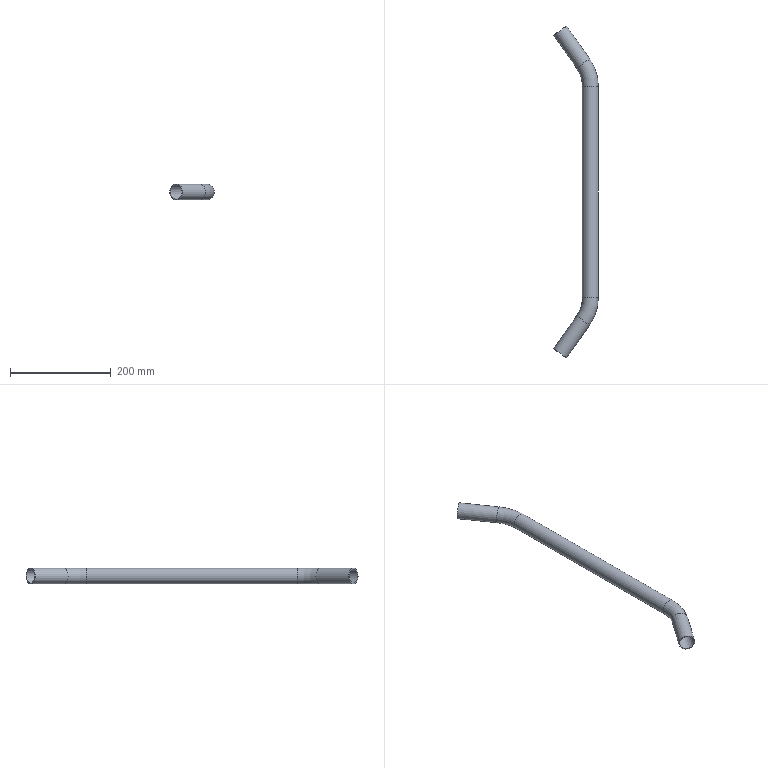Part | STEP file | 7101203 | 1 solid | 12 faces | box 89.278 x 660.628 x 31.8 mm | volume 96707 mm3 | cylinder 6 | torus 4 | plane 2 | commonest cylinder face diameters 28.8 x3 31.8 x3
STEP:
#1=CARTESIAN_POINT('',(0.,0.,0.));
#2=DIRECTION('',(0.,0.,1.));
#3=DIRECTION('',(1.,0.,0.));
#4=AXIS2_PLACEMENT_3D('',#1,#2,#3);
#5=CARTESIAN_POINT('',(-27.492,246.542,0.));
#6=VERTEX_POINT('',#5);
#7=CARTESIAN_POINT('',(-14.468,255.662,0.));
#8=DIRECTION('',(-0.5736,0.8192,0.));
#9=DIRECTION('',(-0.8192,-0.5736,0.));
#10=AXIS2_PLACEMENT_3D('',#7,#8,#9);
#11=CIRCLE('',#10,15.9);
#12=CARTESIAN_POINT('',(-14.468,255.662,0.));
#13=DIRECTION('',(-0.5736,0.8192,0.));
#14=DIRECTION('',(-0.8192,-0.5736,0.));
#15=AXIS2_PLACEMENT_3D('',#12,#13,#14);
#16=CYLINDRICAL_SURFACE('',#15,15.9);
#17=CARTESIAN_POINT('',(0.,0.));
#18=DIRECTION('',(1.,0.));
#19=VECTOR('',#18,1.);
#20=LINE('',#17,#19);
#21=(GEOMETRIC_REPRESENTATION_CONTEXT(2)PARAMETRIC_REPRESENTATION_CONTEXT()REPRESENTATION_CONTEXT('',''));
#22=DEFINITIONAL_REPRESENTATION('',(#20),#21);
#23=PCURVE('',#16,#22);
#24=CARTESIAN_POINT('',(-80.,209.776,0.));
#25=DIRECTION('',(0.,0.,1.));
#26=DIRECTION('',(1.,0.,0.));
#27=AXIS2_PLACEMENT_3D('',#24,#25,#26);
#28=TOROIDAL_SURFACE('',#27,80.,15.9);
#29=CARTESIAN_POINT('',(6.894,9.425));
#30=DIRECTION('',(0.,-1.));
#31=VECTOR('',#30,1.);
#32=LINE('',#29,#31);
#33=(GEOMETRIC_REPRESENTATION_CONTEXT(2)PARAMETRIC_REPRESENTATION_CONTEXT()REPRESENTATION_CONTEXT('',''));
#34=DEFINITIONAL_REPRESENTATION('',(#32),#33);
#35=PCURVE('',#28,#34);
#36=SURFACE_CURVE('',#11,(#23,#35),.PCURVE_S1.);
#37=EDGE_CURVE('',#6,#6,#36,.T.);
#38=ORIENTED_EDGE('',*,*,#37,.T.);
#39=CARTESIAN_POINT('',(-73.378,312.075,0.));
#40=VERTEX_POINT('',#39);
#41=CARTESIAN_POINT('',(-27.492,246.542,0.));
#42=CARTESIAN_POINT('',(-73.378,312.075,0.));
#43=B_SPLINE_CURVE_WITH_KNOTS('',1,(#41,#42),.UNSPECIFIED.,.F.,.F.,(2,2),(0.,80.),.PIECEWISE_BEZIER_KNOTS.);
#44=CARTESIAN_POINT('',(6.283,0.));
#45=DIRECTION('',(0.,1.));
#46=VECTOR('',#45,1.);
#47=LINE('',#44,#46);
#48=(GEOMETRIC_REPRESENTATION_CONTEXT(2)PARAMETRIC_REPRESENTATION_CONTEXT()REPRESENTATION_CONTEXT('',''));
#49=DEFINITIONAL_REPRESENTATION('',(#47),#48);
#50=PCURVE('',#16,#49);
#51=CARTESIAN_POINT('',(0.,0.));
#52=DIRECTION('',(0.,1.));
#53=VECTOR('',#52,1.);
#54=LINE('',#51,#53);
#55=(GEOMETRIC_REPRESENTATION_CONTEXT(2)PARAMETRIC_REPRESENTATION_CONTEXT()REPRESENTATION_CONTEXT('',''));
#56=DEFINITIONAL_REPRESENTATION('',(#54),#55);
#57=PCURVE('',#16,#56);
#58=SEAM_CURVE('',#43,(#50,#57),.PCURVE_S1.);
#59=EDGE_CURVE('',#6,#40,#58,.T.);
#60=ORIENTED_EDGE('',*,*,#59,.T.);
#61=CARTESIAN_POINT('',(-60.354,321.194,0.));
#62=DIRECTION('',(-0.5736,0.8192,0.));
#63=DIRECTION('',(-0.8192,-0.5736,0.));
#64=AXIS2_PLACEMENT_3D('',#61,#62,#63);
#65=CIRCLE('',#64,15.9);
#66=CARTESIAN_POINT('',(0.,80.));
#67=DIRECTION('',(1.,0.));
#68=VECTOR('',#67,1.);
#69=LINE('',#66,#68);
#70=(GEOMETRIC_REPRESENTATION_CONTEXT(2)PARAMETRIC_REPRESENTATION_CONTEXT()REPRESENTATION_CONTEXT('',''));
#71=DEFINITIONAL_REPRESENTATION('',(#69),#70);
#72=PCURVE('',#16,#71);
#73=CARTESIAN_POINT('',(-60.354,321.194,0.));
#74=DIRECTION('',(-0.5736,0.8192,0.));
#75=DIRECTION('',(-0.8192,-0.5736,0.));
#76=AXIS2_PLACEMENT_3D('',#73,#74,#75);
#77=PLANE('',#76);
#78=CARTESIAN_POINT('',(0.,0.));
#79=DIRECTION('',(1.,0.));
#80=AXIS2_PLACEMENT_2D('',#78,#79);
#81=CIRCLE('',#80,15.9);
#82=(GEOMETRIC_REPRESENTATION_CONTEXT(2)PARAMETRIC_REPRESENTATION_CONTEXT()REPRESENTATION_CONTEXT('',''));
#83=DEFINITIONAL_REPRESENTATION('',(#81),#82);
#84=PCURVE('',#77,#83);
#85=SURFACE_CURVE('',#65,(#72,#84),.PCURVE_S1.);
#86=EDGE_CURVE('',#40,#40,#85,.T.);
#87=ORIENTED_EDGE('',*,*,#86,.F.);
#88=ORIENTED_EDGE('',*,*,#59,.F.);
#89=EDGE_LOOP('',(#38,#60,#87,#88));
#90=FACE_BOUND('',#89,.T.);
#91=ADVANCED_FACE('',(#90),#16,.T.);
#92=CARTESIAN_POINT('',(-26.264,247.403,0.));
#93=VERTEX_POINT('',#92);
#94=CARTESIAN_POINT('',(-14.468,255.662,0.));
#95=DIRECTION('',(-0.5736,0.8192,0.));
#96=DIRECTION('',(-0.8192,-0.5736,0.));
#97=AXIS2_PLACEMENT_3D('',#94,#95,#96);
#98=CIRCLE('',#97,14.4);
#99=CARTESIAN_POINT('',(-14.468,255.662,0.));
#100=DIRECTION('',(-0.5736,0.8192,0.));
#101=DIRECTION('',(-0.8192,-0.5736,0.));
#102=AXIS2_PLACEMENT_3D('',#99,#100,#101);
#103=CYLINDRICAL_SURFACE('',#102,14.4);
#104=CARTESIAN_POINT('',(0.,0.));
#105=DIRECTION('',(1.,0.));
#106=VECTOR('',#105,1.);
#107=LINE('',#104,#106);
#108=(GEOMETRIC_REPRESENTATION_CONTEXT(2)PARAMETRIC_REPRESENTATION_CONTEXT()REPRESENTATION_CONTEXT('',''));
#109=DEFINITIONAL_REPRESENTATION('',(#107),#108);
#110=PCURVE('',#103,#109);
#111=CARTESIAN_POINT('',(-80.,209.776,0.));
#112=DIRECTION('',(0.,0.,1.));
#113=DIRECTION('',(1.,0.,0.));
#114=AXIS2_PLACEMENT_3D('',#111,#112,#113);
#115=TOROIDAL_SURFACE('',#114,80.,14.4);
#116=CARTESIAN_POINT('',(6.894,9.425));
#117=DIRECTION('',(0.,-1.));
#118=VECTOR('',#117,1.);
#119=LINE('',#116,#118);
#120=(GEOMETRIC_REPRESENTATION_CONTEXT(2)PARAMETRIC_REPRESENTATION_CONTEXT()REPRESENTATION_CONTEXT('',''));
#121=DEFINITIONAL_REPRESENTATION('',(#119),#120);
#122=PCURVE('',#115,#121);
#123=SURFACE_CURVE('',#98,(#110,#122),.PCURVE_S1.);
#124=EDGE_CURVE('',#93,#93,#123,.T.);
#125=ORIENTED_EDGE('',*,*,#124,.T.);
#126=CARTESIAN_POINT('',(-72.15,312.935,0.));
#127=VERTEX_POINT('',#126);
#128=CARTESIAN_POINT('',(-26.264,247.403,0.));
#129=CARTESIAN_POINT('',(-72.15,312.935,0.));
#130=B_SPLINE_CURVE_WITH_KNOTS('',1,(#128,#129),.UNSPECIFIED.,.F.,.F.,(2,2),(0.,80.),.PIECEWISE_BEZIER_KNOTS.);
#131=CARTESIAN_POINT('',(6.283,0.));
#132=DIRECTION('',(0.,1.));
#133=VECTOR('',#132,1.);
#134=LINE('',#131,#133);
#135=(GEOMETRIC_REPRESENTATION_CONTEXT(2)PARAMETRIC_REPRESENTATION_CONTEXT()REPRESENTATION_CONTEXT('',''));
#136=DEFINITIONAL_REPRESENTATION('',(#134),#135);
#137=PCURVE('',#103,#136);
#138=CARTESIAN_POINT('',(0.,0.));
#139=DIRECTION('',(0.,1.));
#140=VECTOR('',#139,1.);
#141=LINE('',#138,#140);
#142=(GEOMETRIC_REPRESENTATION_CONTEXT(2)PARAMETRIC_REPRESENTATION_CONTEXT()REPRESENTATION_CONTEXT('',''));
#143=DEFINITIONAL_REPRESENTATION('',(#141),#142);
#144=PCURVE('',#103,#143);
#145=SEAM_CURVE('',#130,(#137,#144),.PCURVE_S1.);
#146=EDGE_CURVE('',#93,#127,#145,.T.);
#147=ORIENTED_EDGE('',*,*,#146,.T.);
#148=CARTESIAN_POINT('',(-60.354,321.194,0.));
#149=DIRECTION('',(-0.5736,0.8192,0.));
#150=DIRECTION('',(-0.8192,-0.5736,0.));
#151=AXIS2_PLACEMENT_3D('',#148,#149,#150);
#152=CIRCLE('',#151,14.4);
#153=CARTESIAN_POINT('',(0.,80.));
#154=DIRECTION('',(1.,0.));
#155=VECTOR('',#154,1.);
#156=LINE('',#153,#155);
#157=(GEOMETRIC_REPRESENTATION_CONTEXT(2)PARAMETRIC_REPRESENTATION_CONTEXT()REPRESENTATION_CONTEXT('',''));
#158=DEFINITIONAL_REPRESENTATION('',(#156),#157);
#159=PCURVE('',#103,#158);
#160=CARTESIAN_POINT('',(0.,0.));
#161=DIRECTION('',(1.,0.));
#162=AXIS2_PLACEMENT_2D('',#160,#161);
#163=CIRCLE('',#162,14.4);
#164=(GEOMETRIC_REPRESENTATION_CONTEXT(2)PARAMETRIC_REPRESENTATION_CONTEXT()REPRESENTATION_CONTEXT('',''));
#165=DEFINITIONAL_REPRESENTATION('',(#163),#164);
#166=PCURVE('',#77,#165);
#167=SURFACE_CURVE('',#152,(#159,#166),.PCURVE_S1.);
#168=EDGE_CURVE('',#127,#127,#167,.T.);
#169=ORIENTED_EDGE('',*,*,#168,.F.);
#170=ORIENTED_EDGE('',*,*,#146,.F.);
#171=EDGE_LOOP('',(#125,#147,#169,#170));
#172=FACE_BOUND('',#171,.F.);
#173=ADVANCED_FACE('',(#172),#103,.F.);
#174=CARTESIAN_POINT('',(-15.9,209.776,0.));
#175=VERTEX_POINT('',#174);
#176=CARTESIAN_POINT('',(0.,209.776,0.));
#177=DIRECTION('',(0.,1.,0.));
#178=DIRECTION('',(-1.,0.,0.));
#179=AXIS2_PLACEMENT_3D('',#176,#177,#178);
#180=CIRCLE('',#179,15.9);
#181=CARTESIAN_POINT('',(6.283,9.425));
#182=DIRECTION('',(0.,-1.));
#183=VECTOR('',#182,1.);
#184=LINE('',#181,#183);
#185=(GEOMETRIC_REPRESENTATION_CONTEXT(2)PARAMETRIC_REPRESENTATION_CONTEXT()REPRESENTATION_CONTEXT('',''));
#186=DEFINITIONAL_REPRESENTATION('',(#184),#185);
#187=PCURVE('',#28,#186);
#188=CARTESIAN_POINT('',(0.,-209.776,0.));
#189=DIRECTION('',(0.,1.,0.));
#190=DIRECTION('',(-1.,0.,0.));
#191=AXIS2_PLACEMENT_3D('',#188,#189,#190);
#192=CYLINDRICAL_SURFACE('',#191,15.9);
#193=CARTESIAN_POINT('',(0.,419.552));
#194=DIRECTION('',(1.,0.));
#195=VECTOR('',#194,1.);
#196=LINE('',#193,#195);
#197=(GEOMETRIC_REPRESENTATION_CONTEXT(2)PARAMETRIC_REPRESENTATION_CONTEXT()REPRESENTATION_CONTEXT('',''));
#198=DEFINITIONAL_REPRESENTATION('',(#196),#197);
#199=PCURVE('',#192,#198);
#200=SURFACE_CURVE('',#180,(#187,#199),.PCURVE_S1.);
#201=EDGE_CURVE('',#175,#175,#200,.T.);
#202=ORIENTED_EDGE('',*,*,#201,.T.);
#203=CARTESIAN_POINT('',(-15.9,209.776,0.));
#204=CARTESIAN_POINT('',(-15.9,216.323,0.));
#205=CARTESIAN_POINT('',(-16.701,222.844,0.));
#206=CARTESIAN_POINT('',(-18.294,229.232,0.));
#207=CARTESIAN_POINT('',(-20.653,235.378,0.));
#208=CARTESIAN_POINT('',(-23.737,241.18,0.));
#209=CARTESIAN_POINT('',(-27.492,246.542,0.));
#210=(BOUNDED_CURVE()B_SPLINE_CURVE(6,(#203,#204,#205,#206,#207,#208,#209),.UNSPECIFIED.,.F.,.F.)B_SPLINE_CURVE_WITH_KNOTS((7,7),(6.283,6.894),.PIECEWISE_BEZIER_KNOTS.)CURVE()GEOMETRIC_REPRESENTATION_ITEM()RATIONAL_B_SPLINE_CURVE((1.005,1.002,0.9997,0.9991,0.9997,1.002,1.005))REPRESENTATION_ITEM(''));
#211=CARTESIAN_POINT('',(0.,3.142));
#212=DIRECTION('',(1.,0.));
#213=VECTOR('',#212,1.);
#214=LINE('',#211,#213);
#215=(GEOMETRIC_REPRESENTATION_CONTEXT(2)PARAMETRIC_REPRESENTATION_CONTEXT()REPRESENTATION_CONTEXT('',''));
#216=DEFINITIONAL_REPRESENTATION('',(#214),#215);
#217=PCURVE('',#28,#216);
#218=CARTESIAN_POINT('',(0.,9.425));
#219=DIRECTION('',(1.,0.));
#220=VECTOR('',#219,1.);
#221=LINE('',#218,#220);
#222=(GEOMETRIC_REPRESENTATION_CONTEXT(2)PARAMETRIC_REPRESENTATION_CONTEXT()REPRESENTATION_CONTEXT('',''));
#223=DEFINITIONAL_REPRESENTATION('',(#221),#222);
#224=PCURVE('',#28,#223);
#225=SEAM_CURVE('',#210,(#217,#224),.PCURVE_S1.);
#226=EDGE_CURVE('',#175,#6,#225,.T.);
#227=ORIENTED_EDGE('',*,*,#226,.T.);
#228=ORIENTED_EDGE('',*,*,#37,.F.);
#229=ORIENTED_EDGE('',*,*,#226,.F.);
#230=EDGE_LOOP('',(#202,#227,#228,#229));
#231=FACE_BOUND('',#230,.T.);
#232=ADVANCED_FACE('',(#231),#28,.T.);
#233=CARTESIAN_POINT('',(-14.4,209.776,0.));
#234=VERTEX_POINT('',#233);
#235=CARTESIAN_POINT('',(0.,209.776,0.));
#236=DIRECTION('',(0.,1.,0.));
#237=DIRECTION('',(-1.,0.,0.));
#238=AXIS2_PLACEMENT_3D('',#235,#236,#237);
#239=CIRCLE('',#238,14.4);
#240=CARTESIAN_POINT('',(6.283,9.425));
#241=DIRECTION('',(0.,-1.));
#242=VECTOR('',#241,1.);
#243=LINE('',#240,#242);
#244=(GEOMETRIC_REPRESENTATION_CONTEXT(2)PARAMETRIC_REPRESENTATION_CONTEXT()REPRESENTATION_CONTEXT('',''));
#245=DEFINITIONAL_REPRESENTATION('',(#243),#244);
#246=PCURVE('',#115,#245);
#247=CARTESIAN_POINT('',(0.,-209.776,0.));
#248=DIRECTION('',(0.,1.,0.));
#249=DIRECTION('',(-1.,0.,0.));
#250=AXIS2_PLACEMENT_3D('',#247,#248,#249);
#251=CYLINDRICAL_SURFACE('',#250,14.4);
#252=CARTESIAN_POINT('',(0.,419.552));
#253=DIRECTION('',(1.,0.));
#254=VECTOR('',#253,1.);
#255=LINE('',#252,#254);
#256=(GEOMETRIC_REPRESENTATION_CONTEXT(2)PARAMETRIC_REPRESENTATION_CONTEXT()REPRESENTATION_CONTEXT('',''));
#257=DEFINITIONAL_REPRESENTATION('',(#255),#256);
#258=PCURVE('',#251,#257);
#259=SURFACE_CURVE('',#239,(#246,#258),.PCURVE_S1.);
#260=EDGE_CURVE('',#234,#234,#259,.T.);
#261=ORIENTED_EDGE('',*,*,#260,.T.);
#262=CARTESIAN_POINT('',(-14.4,209.776,0.));
#263=CARTESIAN_POINT('',(-14.4,216.476,0.));
#264=CARTESIAN_POINT('',(-15.22,223.15,0.));
#265=CARTESIAN_POINT('',(-16.85,229.687,0.));
#266=CARTESIAN_POINT('',(-19.264,235.977,0.));
#267=CARTESIAN_POINT('',(-22.421,241.915,0.));
#268=CARTESIAN_POINT('',(-26.264,247.403,0.));
#269=(BOUNDED_CURVE()B_SPLINE_CURVE(6,(#262,#263,#264,#265,#266,#267,#268),.UNSPECIFIED.,.F.,.F.)B_SPLINE_CURVE_WITH_KNOTS((7,7),(6.283,6.894),.PIECEWISE_BEZIER_KNOTS.)CURVE()GEOMETRIC_REPRESENTATION_ITEM()RATIONAL_B_SPLINE_CURVE((1.005,1.002,0.9997,0.9991,0.9997,1.002,1.005))REPRESENTATION_ITEM(''));
#270=CARTESIAN_POINT('',(0.,3.142));
#271=DIRECTION('',(1.,0.));
#272=VECTOR('',#271,1.);
#273=LINE('',#270,#272);
#274=(GEOMETRIC_REPRESENTATION_CONTEXT(2)PARAMETRIC_REPRESENTATION_CONTEXT()REPRESENTATION_CONTEXT('',''));
#275=DEFINITIONAL_REPRESENTATION('',(#273),#274);
#276=PCURVE('',#115,#275);
#277=CARTESIAN_POINT('',(0.,9.425));
#278=DIRECTION('',(1.,0.));
#279=VECTOR('',#278,1.);
#280=LINE('',#277,#279);
#281=(GEOMETRIC_REPRESENTATION_CONTEXT(2)PARAMETRIC_REPRESENTATION_CONTEXT()REPRESENTATION_CONTEXT('',''));
#282=DEFINITIONAL_REPRESENTATION('',(#280),#281);
#283=PCURVE('',#115,#282);
#284=SEAM_CURVE('',#269,(#276,#283),.PCURVE_S1.);
#285=EDGE_CURVE('',#234,#93,#284,.T.);
#286=ORIENTED_EDGE('',*,*,#285,.T.);
#287=ORIENTED_EDGE('',*,*,#124,.F.);
#288=ORIENTED_EDGE('',*,*,#285,.F.);
#289=EDGE_LOOP('',(#261,#286,#287,#288));
#290=FACE_BOUND('',#289,.F.);
#291=ADVANCED_FACE('',(#290),#115,.F.);
#292=CARTESIAN_POINT('',(-15.9,-209.776,0.));
#293=VERTEX_POINT('',#292);
#294=CARTESIAN_POINT('',(0.,-209.776,0.));
#295=DIRECTION('',(0.,1.,0.));
#296=DIRECTION('',(-1.,0.,0.));
#297=AXIS2_PLACEMENT_3D('',#294,#295,#296);
#298=CIRCLE('',#297,15.9);
#299=CARTESIAN_POINT('',(0.,0.));
#300=DIRECTION('',(1.,0.));
#301=VECTOR('',#300,1.);
#302=LINE('',#299,#301);
#303=(GEOMETRIC_REPRESENTATION_CONTEXT(2)PARAMETRIC_REPRESENTATION_CONTEXT()REPRESENTATION_CONTEXT('',''));
#304=DEFINITIONAL_REPRESENTATION('',(#302),#303);
#305=PCURVE('',#192,#304);
#306=CARTESIAN_POINT('',(-80.,-209.776,0.));
#307=DIRECTION('',(0.,0.,1.));
#308=DIRECTION('',(1.,0.,0.));
#309=AXIS2_PLACEMENT_3D('',#306,#307,#308);
#310=TOROIDAL_SURFACE('',#309,80.,15.9);
#311=CARTESIAN_POINT('',(6.283,9.425));
#312=DIRECTION('',(0.,-1.));
#313=VECTOR('',#312,1.);
#314=LINE('',#311,#313);
#315=(GEOMETRIC_REPRESENTATION_CONTEXT(2)PARAMETRIC_REPRESENTATION_CONTEXT()REPRESENTATION_CONTEXT('',''));
#316=DEFINITIONAL_REPRESENTATION('',(#314),#315);
#317=PCURVE('',#310,#316);
#318=SURFACE_CURVE('',#298,(#305,#317),.PCURVE_S1.);
#319=EDGE_CURVE('',#293,#293,#318,.T.);
#320=ORIENTED_EDGE('',*,*,#319,.T.);
#321=CARTESIAN_POINT('',(-15.9,-209.776,0.));
#322=CARTESIAN_POINT('',(-15.9,209.776,0.));
#323=B_SPLINE_CURVE_WITH_KNOTS('',1,(#321,#322),.UNSPECIFIED.,.F.,.F.,(2,2),(0.,419.552),.PIECEWISE_BEZIER_KNOTS.);
#324=CARTESIAN_POINT('',(6.283,0.));
#325=DIRECTION('',(0.,1.));
#326=VECTOR('',#325,1.);
#327=LINE('',#324,#326);
#328=(GEOMETRIC_REPRESENTATION_CONTEXT(2)PARAMETRIC_REPRESENTATION_CONTEXT()REPRESENTATION_CONTEXT('',''));
#329=DEFINITIONAL_REPRESENTATION('',(#327),#328);
#330=PCURVE('',#192,#329);
#331=CARTESIAN_POINT('',(0.,0.));
#332=DIRECTION('',(0.,1.));
#333=VECTOR('',#332,1.);
#334=LINE('',#331,#333);
#335=(GEOMETRIC_REPRESENTATION_CONTEXT(2)PARAMETRIC_REPRESENTATION_CONTEXT()REPRESENTATION_CONTEXT('',''));
#336=DEFINITIONAL_REPRESENTATION('',(#334),#335);
#337=PCURVE('',#192,#336);
#338=SEAM_CURVE('',#323,(#330,#337),.PCURVE_S1.);
#339=EDGE_CURVE('',#293,#175,#338,.T.);
#340=ORIENTED_EDGE('',*,*,#339,.T.);
#341=ORIENTED_EDGE('',*,*,#201,.F.);
#342=ORIENTED_EDGE('',*,*,#339,.F.);
#343=EDGE_LOOP('',(#320,#340,#341,#342));
#344=FACE_BOUND('',#343,.T.);
#345=ADVANCED_FACE('',(#344),#192,.T.);
#346=CARTESIAN_POINT('',(-14.4,-209.776,0.));
#347=VERTEX_POINT('',#346);
#348=CARTESIAN_POINT('',(0.,-209.776,0.));
#349=DIRECTION('',(0.,1.,0.));
#350=DIRECTION('',(-1.,0.,0.));
#351=AXIS2_PLACEMENT_3D('',#348,#349,#350);
#352=CIRCLE('',#351,14.4);
#353=CARTESIAN_POINT('',(0.,0.));
#354=DIRECTION('',(1.,0.));
#355=VECTOR('',#354,1.);
#356=LINE('',#353,#355);
#357=(GEOMETRIC_REPRESENTATION_CONTEXT(2)PARAMETRIC_REPRESENTATION_CONTEXT()REPRESENTATION_CONTEXT('',''));
#358=DEFINITIONAL_REPRESENTATION('',(#356),#357);
#359=PCURVE('',#251,#358);
#360=CARTESIAN_POINT('',(-80.,-209.776,0.));
#361=DIRECTION('',(0.,0.,1.));
#362=DIRECTION('',(1.,0.,0.));
#363=AXIS2_PLACEMENT_3D('',#360,#361,#362);
#364=TOROIDAL_SURFACE('',#363,80.,14.4);
#365=CARTESIAN_POINT('',(6.283,9.425));
#366=DIRECTION('',(0.,-1.));
#367=VECTOR('',#366,1.);
#368=LINE('',#365,#367);
#369=(GEOMETRIC_REPRESENTATION_CONTEXT(2)PARAMETRIC_REPRESENTATION_CONTEXT()REPRESENTATION_CONTEXT('',''));
#370=DEFINITIONAL_REPRESENTATION('',(#368),#369);
#371=PCURVE('',#364,#370);
#372=SURFACE_CURVE('',#352,(#359,#371),.PCURVE_S1.);
#373=EDGE_CURVE('',#347,#347,#372,.T.);
#374=ORIENTED_EDGE('',*,*,#373,.T.);
#375=CARTESIAN_POINT('',(-14.4,-209.776,0.));
#376=CARTESIAN_POINT('',(-14.4,209.776,0.));
#377=B_SPLINE_CURVE_WITH_KNOTS('',1,(#375,#376),.UNSPECIFIED.,.F.,.F.,(2,2),(0.,419.552),.PIECEWISE_BEZIER_KNOTS.);
#378=CARTESIAN_POINT('',(6.283,0.));
#379=DIRECTION('',(0.,1.));
#380=VECTOR('',#379,1.);
#381=LINE('',#378,#380);
#382=(GEOMETRIC_REPRESENTATION_CONTEXT(2)PARAMETRIC_REPRESENTATION_CONTEXT()REPRESENTATION_CONTEXT('',''));
#383=DEFINITIONAL_REPRESENTATION('',(#381),#382);
#384=PCURVE('',#251,#383);
#385=CARTESIAN_POINT('',(0.,0.));
#386=DIRECTION('',(0.,1.));
#387=VECTOR('',#386,1.);
#388=LINE('',#385,#387);
#389=(GEOMETRIC_REPRESENTATION_CONTEXT(2)PARAMETRIC_REPRESENTATION_CONTEXT()REPRESENTATION_CONTEXT('',''));
#390=DEFINITIONAL_REPRESENTATION('',(#388),#389);
#391=PCURVE('',#251,#390);
#392=SEAM_CURVE('',#377,(#384,#391),.PCURVE_S1.);
#393=EDGE_CURVE('',#347,#234,#392,.T.);
#394=ORIENTED_EDGE('',*,*,#393,.T.);
#395=ORIENTED_EDGE('',*,*,#260,.F.);
#396=ORIENTED_EDGE('',*,*,#393,.F.);
#397=EDGE_LOOP('',(#374,#394,#395,#396));
#398=FACE_BOUND('',#397,.F.);
#399=ADVANCED_FACE('',(#398),#251,.F.);
#400=CARTESIAN_POINT('',(-27.492,-246.542,0.));
#401=VERTEX_POINT('',#400);
#402=CARTESIAN_POINT('',(-14.468,-255.662,0.));
#403=DIRECTION('',(0.5736,0.8192,0.));
#404=DIRECTION('',(-0.8192,0.5736,0.));
#405=AXIS2_PLACEMENT_3D('',#402,#403,#404);
#406=CIRCLE('',#405,15.9);
#407=CARTESIAN_POINT('',(5.672,9.425));
#408=DIRECTION('',(0.,-1.));
#409=VECTOR('',#408,1.);
#410=LINE('',#407,#409);
#411=(GEOMETRIC_REPRESENTATION_CONTEXT(2)PARAMETRIC_REPRESENTATION_CONTEXT()REPRESENTATION_CONTEXT('',''));
#412=DEFINITIONAL_REPRESENTATION('',(#410),#411);
#413=PCURVE('',#310,#412);
#414=CARTESIAN_POINT('',(-14.468,-255.662,0.));
#415=DIRECTION('',(-0.5736,-0.8192,0.));
#416=DIRECTION('',(0.8192,-0.5736,0.));
#417=AXIS2_PLACEMENT_3D('',#414,#415,#416);
#418=CYLINDRICAL_SURFACE('',#417,15.9);
#419=CARTESIAN_POINT('',(9.425,0.));
#420=DIRECTION('',(-1.,0.));
#421=VECTOR('',#420,1.);
#422=LINE('',#419,#421);
#423=(GEOMETRIC_REPRESENTATION_CONTEXT(2)PARAMETRIC_REPRESENTATION_CONTEXT()REPRESENTATION_CONTEXT('',''));
#424=DEFINITIONAL_REPRESENTATION('',(#422),#423);
#425=PCURVE('',#418,#424);
#426=SURFACE_CURVE('',#406,(#413,#425),.PCURVE_S1.);
#427=EDGE_CURVE('',#401,#401,#426,.T.);
#428=ORIENTED_EDGE('',*,*,#427,.T.);
#429=CARTESIAN_POINT('',(-27.492,-246.542,0.));
#430=CARTESIAN_POINT('',(-23.737,-241.18,0.));
#431=CARTESIAN_POINT('',(-20.653,-235.378,0.));
#432=CARTESIAN_POINT('',(-18.294,-229.232,0.));
#433=CARTESIAN_POINT('',(-16.701,-222.844,0.));
#434=CARTESIAN_POINT('',(-15.9,-216.323,0.));
#435=CARTESIAN_POINT('',(-15.9,-209.776,0.));
#436=(BOUNDED_CURVE()B_SPLINE_CURVE(6,(#429,#430,#431,#432,#433,#434,#435),.UNSPECIFIED.,.F.,.F.)B_SPLINE_CURVE_WITH_KNOTS((7,7),(5.672,6.283),.PIECEWISE_BEZIER_KNOTS.)CURVE()GEOMETRIC_REPRESENTATION_ITEM()RATIONAL_B_SPLINE_CURVE((1.005,1.002,0.9997,0.9991,0.9997,1.002,1.005))REPRESENTATION_ITEM(''));
#437=CARTESIAN_POINT('',(0.,3.142));
#438=DIRECTION('',(1.,0.));
#439=VECTOR('',#438,1.);
#440=LINE('',#437,#439);
#441=(GEOMETRIC_REPRESENTATION_CONTEXT(2)PARAMETRIC_REPRESENTATION_CONTEXT()REPRESENTATION_CONTEXT('',''));
#442=DEFINITIONAL_REPRESENTATION('',(#440),#441);
#443=PCURVE('',#310,#442);
#444=CARTESIAN_POINT('',(0.,9.425));
#445=DIRECTION('',(1.,0.));
#446=VECTOR('',#445,1.);
#447=LINE('',#444,#446);
#448=(GEOMETRIC_REPRESENTATION_CONTEXT(2)PARAMETRIC_REPRESENTATION_CONTEXT()REPRESENTATION_CONTEXT('',''));
#449=DEFINITIONAL_REPRESENTATION('',(#447),#448);
#450=PCURVE('',#310,#449);
#451=SEAM_CURVE('',#436,(#443,#450),.PCURVE_S1.);
#452=EDGE_CURVE('',#401,#293,#451,.T.);
#453=ORIENTED_EDGE('',*,*,#452,.T.);
#454=ORIENTED_EDGE('',*,*,#319,.F.);
#455=ORIENTED_EDGE('',*,*,#452,.F.);
#456=EDGE_LOOP('',(#428,#453,#454,#455));
#457=FACE_BOUND('',#456,.T.);
#458=ADVANCED_FACE('',(#457),#310,.T.);
#459=CARTESIAN_POINT('',(-26.264,-247.403,0.));
#460=VERTEX_POINT('',#459);
#461=CARTESIAN_POINT('',(-14.468,-255.662,0.));
#462=DIRECTION('',(0.5736,0.8192,0.));
#463=DIRECTION('',(-0.8192,0.5736,0.));
#464=AXIS2_PLACEMENT_3D('',#461,#462,#463);
#465=CIRCLE('',#464,14.4);
#466=CARTESIAN_POINT('',(5.672,9.425));
#467=DIRECTION('',(0.,-1.));
#468=VECTOR('',#467,1.);
#469=LINE('',#466,#468);
#470=(GEOMETRIC_REPRESENTATION_CONTEXT(2)PARAMETRIC_REPRESENTATION_CONTEXT()REPRESENTATION_CONTEXT('',''));
#471=DEFINITIONAL_REPRESENTATION('',(#469),#470);
#472=PCURVE('',#364,#471);
#473=CARTESIAN_POINT('',(-14.468,-255.662,0.));
#474=DIRECTION('',(-0.5736,-0.8192,0.));
#475=DIRECTION('',(0.8192,-0.5736,0.));
#476=AXIS2_PLACEMENT_3D('',#473,#474,#475);
#477=CYLINDRICAL_SURFACE('',#476,14.4);
#478=CARTESIAN_POINT('',(9.425,0.));
#479=DIRECTION('',(-1.,0.));
#480=VECTOR('',#479,1.);
#481=LINE('',#478,#480);
#482=(GEOMETRIC_REPRESENTATION_CONTEXT(2)PARAMETRIC_REPRESENTATION_CONTEXT()REPRESENTATION_CONTEXT('',''));
#483=DEFINITIONAL_REPRESENTATION('',(#481),#482);
#484=PCURVE('',#477,#483);
#485=SURFACE_CURVE('',#465,(#472,#484),.PCURVE_S1.);
#486=EDGE_CURVE('',#460,#460,#485,.T.);
#487=ORIENTED_EDGE('',*,*,#486,.T.);
#488=CARTESIAN_POINT('',(-26.264,-247.403,0.));
#489=CARTESIAN_POINT('',(-22.421,-241.915,0.));
#490=CARTESIAN_POINT('',(-19.264,-235.977,0.));
#491=CARTESIAN_POINT('',(-16.85,-229.687,0.));
#492=CARTESIAN_POINT('',(-15.22,-223.15,0.));
#493=CARTESIAN_POINT('',(-14.4,-216.476,0.));
#494=CARTESIAN_POINT('',(-14.4,-209.776,0.));
#495=(BOUNDED_CURVE()B_SPLINE_CURVE(6,(#488,#489,#490,#491,#492,#493,#494),.UNSPECIFIED.,.F.,.F.)B_SPLINE_CURVE_WITH_KNOTS((7,7),(5.672,6.283),.PIECEWISE_BEZIER_KNOTS.)CURVE()GEOMETRIC_REPRESENTATION_ITEM()RATIONAL_B_SPLINE_CURVE((1.005,1.002,0.9997,0.9991,0.9997,1.002,1.005))REPRESENTATION_ITEM(''));
#496=CARTESIAN_POINT('',(0.,3.142));
#497=DIRECTION('',(1.,0.));
#498=VECTOR('',#497,1.);
#499=LINE('',#496,#498);
#500=(GEOMETRIC_REPRESENTATION_CONTEXT(2)PARAMETRIC_REPRESENTATION_CONTEXT()REPRESENTATION_CONTEXT('',''));
#501=DEFINITIONAL_REPRESENTATION('',(#499),#500);
#502=PCURVE('',#364,#501);
#503=CARTESIAN_POINT('',(0.,9.425));
#504=DIRECTION('',(1.,0.));
#505=VECTOR('',#504,1.);
#506=LINE('',#503,#505);
#507=(GEOMETRIC_REPRESENTATION_CONTEXT(2)PARAMETRIC_REPRESENTATION_CONTEXT()REPRESENTATION_CONTEXT('',''));
#508=DEFINITIONAL_REPRESENTATION('',(#506),#507);
#509=PCURVE('',#364,#508);
#510=SEAM_CURVE('',#495,(#502,#509),.PCURVE_S1.);
#511=EDGE_CURVE('',#460,#347,#510,.T.);
#512=ORIENTED_EDGE('',*,*,#511,.T.);
#513=ORIENTED_EDGE('',*,*,#373,.F.);
#514=ORIENTED_EDGE('',*,*,#511,.F.);
#515=EDGE_LOOP('',(#487,#512,#513,#514));
#516=FACE_BOUND('',#515,.F.);
#517=ADVANCED_FACE('',(#516),#364,.F.);
#518=ORIENTED_EDGE('',*,*,#486,.F.);
#519=CARTESIAN_POINT('',(-72.15,-312.935,0.));
#520=VERTEX_POINT('',#519);
#521=CARTESIAN_POINT('',(-26.264,-247.403,0.));
#522=CARTESIAN_POINT('',(-72.15,-312.935,0.));
#523=B_SPLINE_CURVE_WITH_KNOTS('',1,(#521,#522),.UNSPECIFIED.,.F.,.F.,(2,2),(0.,80.),.PIECEWISE_BEZIER_KNOTS.);
#524=CARTESIAN_POINT('',(9.425,0.));
#525=DIRECTION('',(0.,1.));
#526=VECTOR('',#525,1.);
#527=LINE('',#524,#526);
#528=(GEOMETRIC_REPRESENTATION_CONTEXT(2)PARAMETRIC_REPRESENTATION_CONTEXT()REPRESENTATION_CONTEXT('',''));
#529=DEFINITIONAL_REPRESENTATION('',(#527),#528);
#530=PCURVE('',#477,#529);
#531=CARTESIAN_POINT('',(3.142,0.));
#532=DIRECTION('',(0.,1.));
#533=VECTOR('',#532,1.);
#534=LINE('',#531,#533);
#535=(GEOMETRIC_REPRESENTATION_CONTEXT(2)PARAMETRIC_REPRESENTATION_CONTEXT()REPRESENTATION_CONTEXT('',''));
#536=DEFINITIONAL_REPRESENTATION('',(#534),#535);
#537=PCURVE('',#477,#536);
#538=SEAM_CURVE('',#523,(#530,#537),.PCURVE_S1.);
#539=EDGE_CURVE('',#460,#520,#538,.T.);
#540=ORIENTED_EDGE('',*,*,#539,.T.);
#541=CARTESIAN_POINT('',(-60.354,-321.194,0.));
#542=DIRECTION('',(0.5736,0.8192,0.));
#543=DIRECTION('',(-0.8192,0.5736,0.));
#544=AXIS2_PLACEMENT_3D('',#541,#542,#543);
#545=CIRCLE('',#544,14.4);
#546=CARTESIAN_POINT('',(9.425,80.));
#547=DIRECTION('',(-1.,0.));
#548=VECTOR('',#547,1.);
#549=LINE('',#546,#548);
#550=(GEOMETRIC_REPRESENTATION_CONTEXT(2)PARAMETRIC_REPRESENTATION_CONTEXT()REPRESENTATION_CONTEXT('',''));
#551=DEFINITIONAL_REPRESENTATION('',(#549),#550);
#552=PCURVE('',#477,#551);
#553=CARTESIAN_POINT('',(-60.354,-321.194,0.));
#554=DIRECTION('',(0.5736,0.8192,0.));
#555=DIRECTION('',(-0.8192,0.5736,0.));
#556=AXIS2_PLACEMENT_3D('',#553,#554,#555);
#557=PLANE('',#556);
#558=CARTESIAN_POINT('',(0.,0.));
#559=DIRECTION('',(1.,0.));
#560=AXIS2_PLACEMENT_2D('',#558,#559);
#561=CIRCLE('',#560,14.4);
#562=(GEOMETRIC_REPRESENTATION_CONTEXT(2)PARAMETRIC_REPRESENTATION_CONTEXT()REPRESENTATION_CONTEXT('',''));
#563=DEFINITIONAL_REPRESENTATION('',(#561),#562);
#564=PCURVE('',#557,#563);
#565=SURFACE_CURVE('',#545,(#552,#564),.PCURVE_S1.);
#566=EDGE_CURVE('',#520,#520,#565,.T.);
#567=ORIENTED_EDGE('',*,*,#566,.T.);
#568=ORIENTED_EDGE('',*,*,#539,.F.);
#569=EDGE_LOOP('',(#518,#540,#567,#568));
#570=FACE_BOUND('',#569,.F.);
#571=ADVANCED_FACE('',(#570),#477,.F.);
#572=ORIENTED_EDGE('',*,*,#427,.F.);
#573=CARTESIAN_POINT('',(-73.378,-312.075,0.));
#574=VERTEX_POINT('',#573);
#575=CARTESIAN_POINT('',(-27.492,-246.542,0.));
#576=CARTESIAN_POINT('',(-73.378,-312.075,0.));
#577=B_SPLINE_CURVE_WITH_KNOTS('',1,(#575,#576),.UNSPECIFIED.,.F.,.F.,(2,2),(0.,80.),.PIECEWISE_BEZIER_KNOTS.);
#578=CARTESIAN_POINT('',(9.425,0.));
#579=DIRECTION('',(0.,1.));
#580=VECTOR('',#579,1.);
#581=LINE('',#578,#580);
#582=(GEOMETRIC_REPRESENTATION_CONTEXT(2)PARAMETRIC_REPRESENTATION_CONTEXT()REPRESENTATION_CONTEXT('',''));
#583=DEFINITIONAL_REPRESENTATION('',(#581),#582);
#584=PCURVE('',#418,#583);
#585=CARTESIAN_POINT('',(3.142,0.));
#586=DIRECTION('',(0.,1.));
#587=VECTOR('',#586,1.);
#588=LINE('',#585,#587);
#589=(GEOMETRIC_REPRESENTATION_CONTEXT(2)PARAMETRIC_REPRESENTATION_CONTEXT()REPRESENTATION_CONTEXT('',''));
#590=DEFINITIONAL_REPRESENTATION('',(#588),#589);
#591=PCURVE('',#418,#590);
#592=SEAM_CURVE('',#577,(#584,#591),.PCURVE_S1.);
#593=EDGE_CURVE('',#401,#574,#592,.T.);
#594=ORIENTED_EDGE('',*,*,#593,.T.);
#595=CARTESIAN_POINT('',(-60.354,-321.194,0.));
#596=DIRECTION('',(0.5736,0.8192,0.));
#597=DIRECTION('',(-0.8192,0.5736,0.));
#598=AXIS2_PLACEMENT_3D('',#595,#596,#597);
#599=CIRCLE('',#598,15.9);
#600=CARTESIAN_POINT('',(9.425,80.));
#601=DIRECTION('',(-1.,0.));
#602=VECTOR('',#601,1.);
#603=LINE('',#600,#602);
#604=(GEOMETRIC_REPRESENTATION_CONTEXT(2)PARAMETRIC_REPRESENTATION_CONTEXT()REPRESENTATION_CONTEXT('',''));
#605=DEFINITIONAL_REPRESENTATION('',(#603),#604);
#606=PCURVE('',#418,#605);
#607=CARTESIAN_POINT('',(0.,0.));
#608=DIRECTION('',(1.,0.));
#609=AXIS2_PLACEMENT_2D('',#607,#608);
#610=CIRCLE('',#609,15.9);
#611=(GEOMETRIC_REPRESENTATION_CONTEXT(2)PARAMETRIC_REPRESENTATION_CONTEXT()REPRESENTATION_CONTEXT('',''));
#612=DEFINITIONAL_REPRESENTATION('',(#610),#611);
#613=PCURVE('',#557,#612);
#614=SURFACE_CURVE('',#599,(#606,#613),.PCURVE_S1.);
#615=EDGE_CURVE('',#574,#574,#614,.T.);
#616=ORIENTED_EDGE('',*,*,#615,.T.);
#617=ORIENTED_EDGE('',*,*,#593,.F.);
#618=EDGE_LOOP('',(#572,#594,#616,#617));
#619=FACE_BOUND('',#618,.T.);
#620=ADVANCED_FACE('',(#619),#418,.T.);
#621=ORIENTED_EDGE('',*,*,#168,.F.);
#622=EDGE_LOOP('',(#621));
#623=FACE_BOUND('',#622,.T.);
#624=ORIENTED_EDGE('',*,*,#86,.T.);
#625=EDGE_LOOP('',(#624));
#626=FACE_BOUND('',#625,.T.);
#627=ADVANCED_FACE('',(#623,#626),#77,.T.);
#628=ORIENTED_EDGE('',*,*,#566,.T.);
#629=EDGE_LOOP('',(#628));
#630=FACE_BOUND('',#629,.T.);
#631=ORIENTED_EDGE('',*,*,#615,.F.);
#632=EDGE_LOOP('',(#631));
#633=FACE_BOUND('',#632,.T.);
#634=ADVANCED_FACE('',(#630,#633),#557,.F.);
#635=CLOSED_SHELL('',(#91,#173,#232,#291,#345,#399,#458,#517,#571,#620,#627,#634));
#636=MANIFOLD_SOLID_BREP('',#635);
#637=(LENGTH_UNIT()NAMED_UNIT(*)SI_UNIT(.MILLI.,.METRE.));
#638=UNCERTAINTY_MEASURE_WITH_UNIT(LENGTH_MEASURE(0.00001),#637,'','');
#639=(NAMED_UNIT(*)PLANE_ANGLE_UNIT()SI_UNIT($,.RADIAN.));
#640=(NAMED_UNIT(*)SI_UNIT($,.STERADIAN.)SOLID_ANGLE_UNIT());
#641=(GEOMETRIC_REPRESENTATION_CONTEXT(3)GLOBAL_UNCERTAINTY_ASSIGNED_CONTEXT((#638))GLOBAL_UNIT_ASSIGNED_CONTEXT((#637,#639,#640))REPRESENTATION_CONTEXT('',''));
#642=ADVANCED_BREP_SHAPE_REPRESENTATION('',(#4,#636),#641);